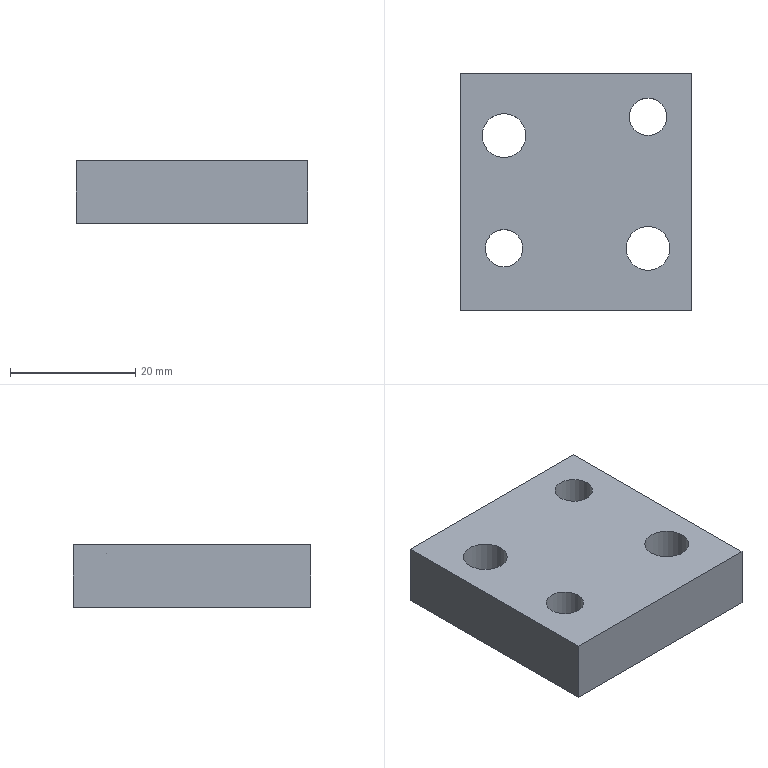Part | NX | features DIE-34 2 | 1 solid | 10 faces | box 37 x 38 x 10 mm | volume 12723 mm3 | plane 6 | cylinder 4 | commonest cylinder face diameters 6 x2 7.009 x2
STEP:
#1=CARTESIAN_POINT('',(2445.569,-956.622,868.716));
#2=VERTEX_POINT('',#1);
#3=CARTESIAN_POINT('',(2482.569,-956.622,868.716));
#4=VERTEX_POINT('',#3);
#5=CARTESIAN_POINT('',(2529.569,-956.622,868.716));
#6=DIRECTION('',(1.,0.,0.));
#7=VECTOR('',#6,1000.);
#8=LINE('',#5,#7);
#9=EDGE_CURVE('',#2,#4,#8,.T.);
#10=ORIENTED_EDGE('',*,*,#9,.T.);
#11=CARTESIAN_POINT('',(2482.569,-956.622,858.716));
#12=VERTEX_POINT('',#11);
#13=CARTESIAN_POINT('',(2482.569,-956.622,858.716));
#14=DIRECTION('',(0.,0.,1.));
#15=VECTOR('',#14,1000.);
#16=LINE('',#13,#15);
#17=EDGE_CURVE('',#4,#12,#16,.F.);
#18=ORIENTED_EDGE('',*,*,#17,.T.);
#19=CARTESIAN_POINT('',(2445.569,-956.622,858.716));
#20=VERTEX_POINT('',#19);
#21=CARTESIAN_POINT('',(2464.069,-956.622,858.716));
#22=DIRECTION('',(1.,0.,0.));
#23=VECTOR('',#22,1000.);
#24=LINE('',#21,#23);
#25=EDGE_CURVE('',#20,#12,#24,.T.);
#26=ORIENTED_EDGE('',*,*,#25,.F.);
#27=CARTESIAN_POINT('',(2445.569,-956.622,858.716));
#28=DIRECTION('',(0.,0.,1.));
#29=VECTOR('',#28,1000.);
#30=LINE('',#27,#29);
#31=EDGE_CURVE('',#20,#2,#30,.T.);
#32=ORIENTED_EDGE('',*,*,#31,.T.);
#33=EDGE_LOOP('',(#10,#18,#26,#32));
#34=FACE_BOUND('',#33,.T.);
#35=CARTESIAN_POINT('',(2464.069,-956.622,858.716));
#36=DIRECTION('',(0.,-1.,0.));
#37=DIRECTION('',(0.,0.,-1.));
#38=AXIS2_PLACEMENT_3D('',#35,#36,#37);
#39=PLANE('',#38);
#40=ADVANCED_FACE('',(#34),#39,.F.);
#41=CARTESIAN_POINT('',(2445.569,-994.622,868.716));
#42=VERTEX_POINT('',#41);
#43=CARTESIAN_POINT('',(2482.569,-994.622,868.716));
#44=VERTEX_POINT('',#43);
#45=CARTESIAN_POINT('',(2529.569,-994.622,868.716));
#46=DIRECTION('',(1.,0.,0.));
#47=VECTOR('',#46,1000.);
#48=LINE('',#45,#47);
#49=EDGE_CURVE('',#42,#44,#48,.T.);
#50=ORIENTED_EDGE('',*,*,#49,.F.);
#51=CARTESIAN_POINT('',(2445.569,-994.622,858.716));
#52=VERTEX_POINT('',#51);
#53=CARTESIAN_POINT('',(2445.569,-994.622,858.716));
#54=DIRECTION('',(0.,0.,1.));
#55=VECTOR('',#54,1000.);
#56=LINE('',#53,#55);
#57=EDGE_CURVE('',#52,#42,#56,.T.);
#58=ORIENTED_EDGE('',*,*,#57,.F.);
#59=CARTESIAN_POINT('',(2482.569,-994.622,858.716));
#60=VERTEX_POINT('',#59);
#61=CARTESIAN_POINT('',(2529.569,-994.622,858.716));
#62=DIRECTION('',(1.,0.,0.));
#63=VECTOR('',#62,1000.);
#64=LINE('',#61,#63);
#65=EDGE_CURVE('',#52,#60,#64,.T.);
#66=ORIENTED_EDGE('',*,*,#65,.T.);
#67=CARTESIAN_POINT('',(2482.569,-994.622,858.716));
#68=DIRECTION('',(0.,0.,1.));
#69=VECTOR('',#68,1000.);
#70=LINE('',#67,#69);
#71=EDGE_CURVE('',#44,#60,#70,.F.);
#72=ORIENTED_EDGE('',*,*,#71,.F.);
#73=EDGE_LOOP('',(#50,#58,#66,#72));
#74=FACE_BOUND('',#73,.T.);
#75=CARTESIAN_POINT('',(2529.569,-994.622,858.716));
#76=DIRECTION('',(0.,-1.,0.));
#77=DIRECTION('',(1.,0.,0.));
#78=AXIS2_PLACEMENT_3D('',#75,#76,#77);
#79=PLANE('',#78);
#80=ADVANCED_FACE('',(#74),#79,.T.);
#81=CARTESIAN_POINT('',(2456.073,-966.622,858.716));
#82=VERTEX_POINT('',#81);
#83=CARTESIAN_POINT('',(2452.569,-966.622,858.716));
#84=DIRECTION('',(0.,0.,1.));
#85=DIRECTION('',(1.,0.,0.));
#86=AXIS2_PLACEMENT_3D('',#83,#84,#85);
#87=CIRCLE('',#86,3.505);
#88=EDGE_CURVE('',#82,#82,#87,.T.);
#89=ORIENTED_EDGE('',*,*,#88,.F.);
#90=EDGE_LOOP('',(#89));
#91=FACE_BOUND('',#90,.T.);
#92=CARTESIAN_POINT('',(2456.073,-966.622,868.716));
#93=VERTEX_POINT('',#92);
#94=CARTESIAN_POINT('',(2452.569,-966.622,868.716));
#95=DIRECTION('',(0.,0.,1.));
#96=DIRECTION('',(1.,0.,0.));
#97=AXIS2_PLACEMENT_3D('',#94,#95,#96);
#98=CIRCLE('',#97,3.505);
#99=EDGE_CURVE('',#93,#93,#98,.T.);
#100=ORIENTED_EDGE('',*,*,#99,.T.);
#101=EDGE_LOOP('',(#100));
#102=FACE_BOUND('',#101,.T.);
#103=CARTESIAN_POINT('',(2452.569,-966.622,858.716));
#104=DIRECTION('',(0.,0.,1.));
#105=DIRECTION('',(1.,0.,0.));
#106=AXIS2_PLACEMENT_3D('',#103,#104,#105);
#107=CYLINDRICAL_SURFACE('',#106,3.505);
#108=ADVANCED_FACE('',(#91,#102),#107,.F.);
#109=CARTESIAN_POINT('',(2455.569,-984.622,858.716));
#110=VERTEX_POINT('',#109);
#111=CARTESIAN_POINT('',(2452.569,-984.622,858.716));
#112=DIRECTION('',(0.,0.,1.));
#113=DIRECTION('',(1.,0.,0.));
#114=AXIS2_PLACEMENT_3D('',#111,#112,#113);
#115=CIRCLE('',#114,3.);
#116=EDGE_CURVE('',#110,#110,#115,.T.);
#117=ORIENTED_EDGE('',*,*,#116,.F.);
#118=EDGE_LOOP('',(#117));
#119=FACE_BOUND('',#118,.T.);
#120=CARTESIAN_POINT('',(2455.569,-984.622,868.716));
#121=VERTEX_POINT('',#120);
#122=CARTESIAN_POINT('',(2452.569,-984.622,868.716));
#123=DIRECTION('',(0.,0.,1.));
#124=DIRECTION('',(1.,0.,0.));
#125=AXIS2_PLACEMENT_3D('',#122,#123,#124);
#126=CIRCLE('',#125,3.);
#127=EDGE_CURVE('',#121,#121,#126,.T.);
#128=ORIENTED_EDGE('',*,*,#127,.T.);
#129=EDGE_LOOP('',(#128));
#130=FACE_BOUND('',#129,.T.);
#131=CARTESIAN_POINT('',(2452.569,-984.622,858.716));
#132=DIRECTION('',(0.,0.,1.));
#133=DIRECTION('',(1.,0.,0.));
#134=AXIS2_PLACEMENT_3D('',#131,#132,#133);
#135=CYLINDRICAL_SURFACE('',#134,3.);
#136=ADVANCED_FACE('',(#119,#130),#135,.F.);
#137=CARTESIAN_POINT('',(2445.569,-849.622,868.716));
#138=DIRECTION('',(0.,1.,0.));
#139=VECTOR('',#138,1000.);
#140=LINE('',#137,#139);
#141=EDGE_CURVE('',#42,#2,#140,.T.);
#142=ORIENTED_EDGE('',*,*,#141,.T.);
#143=ORIENTED_EDGE('',*,*,#31,.F.);
#144=CARTESIAN_POINT('',(2445.569,-989.622,858.716));
#145=DIRECTION('',(0.,1.,0.));
#146=VECTOR('',#145,1000.);
#147=LINE('',#144,#146);
#148=EDGE_CURVE('',#52,#20,#147,.T.);
#149=ORIENTED_EDGE('',*,*,#148,.F.);
#150=ORIENTED_EDGE('',*,*,#57,.T.);
#151=EDGE_LOOP('',(#142,#143,#149,#150));
#152=FACE_BOUND('',#151,.T.);
#153=CARTESIAN_POINT('',(2445.569,-989.622,858.716));
#154=DIRECTION('',(1.,0.,0.));
#155=DIRECTION('',(0.,0.,-1.));
#156=AXIS2_PLACEMENT_3D('',#153,#154,#155);
#157=PLANE('',#156);
#158=ADVANCED_FACE('',(#152),#157,.F.);
#159=ORIENTED_EDGE('',*,*,#116,.T.);
#160=EDGE_LOOP('',(#159));
#161=FACE_BOUND('',#160,.T.);
#162=ORIENTED_EDGE('',*,*,#88,.T.);
#163=EDGE_LOOP('',(#162));
#164=FACE_BOUND('',#163,.T.);
#165=ORIENTED_EDGE('',*,*,#25,.T.);
#166=CARTESIAN_POINT('',(2482.569,-989.622,858.716));
#167=DIRECTION('',(0.,-1.,0.));
#168=VECTOR('',#167,1000.);
#169=LINE('',#166,#168);
#170=EDGE_CURVE('',#60,#12,#169,.F.);
#171=ORIENTED_EDGE('',*,*,#170,.F.);
#172=ORIENTED_EDGE('',*,*,#65,.F.);
#173=ORIENTED_EDGE('',*,*,#148,.T.);
#174=EDGE_LOOP('',(#165,#171,#172,#173));
#175=FACE_BOUND('',#174,.T.);
#176=CARTESIAN_POINT('',(2478.569,-963.622,858.716));
#177=VERTEX_POINT('',#176);
#178=CARTESIAN_POINT('',(2475.569,-963.622,858.716));
#179=DIRECTION('',(0.,0.,1.));
#180=DIRECTION('',(1.,0.,0.));
#181=AXIS2_PLACEMENT_3D('',#178,#179,#180);
#182=CIRCLE('',#181,3.);
#183=EDGE_CURVE('',#177,#177,#182,.F.);
#184=ORIENTED_EDGE('',*,*,#183,.F.);
#185=EDGE_LOOP('',(#184));
#186=FACE_BOUND('',#185,.T.);
#187=CARTESIAN_POINT('',(2479.073,-984.622,858.716));
#188=VERTEX_POINT('',#187);
#189=CARTESIAN_POINT('',(2475.569,-984.622,858.716));
#190=DIRECTION('',(0.,0.,1.));
#191=DIRECTION('',(1.,0.,0.));
#192=AXIS2_PLACEMENT_3D('',#189,#190,#191);
#193=CIRCLE('',#192,3.505);
#194=EDGE_CURVE('',#188,#188,#193,.F.);
#195=ORIENTED_EDGE('',*,*,#194,.F.);
#196=EDGE_LOOP('',(#195));
#197=FACE_BOUND('',#196,.T.);
#198=CARTESIAN_POINT('',(2529.569,-849.622,858.716));
#199=DIRECTION('',(0.,0.,1.));
#200=DIRECTION('',(-1.,0.,0.));
#201=AXIS2_PLACEMENT_3D('',#198,#199,#200);
#202=PLANE('',#201);
#203=ADVANCED_FACE('',(#161,#164,#175,#186,#197),#202,.F.);
#204=ORIENTED_EDGE('',*,*,#127,.F.);
#205=EDGE_LOOP('',(#204));
#206=FACE_BOUND('',#205,.T.);
#207=ORIENTED_EDGE('',*,*,#99,.F.);
#208=EDGE_LOOP('',(#207));
#209=FACE_BOUND('',#208,.T.);
#210=ORIENTED_EDGE('',*,*,#9,.F.);
#211=ORIENTED_EDGE('',*,*,#141,.F.);
#212=ORIENTED_EDGE('',*,*,#49,.T.);
#213=CARTESIAN_POINT('',(2482.569,-989.622,868.716));
#214=DIRECTION('',(0.,1.,0.));
#215=VECTOR('',#214,1000.);
#216=LINE('',#213,#215);
#217=EDGE_CURVE('',#44,#4,#216,.T.);
#218=ORIENTED_EDGE('',*,*,#217,.T.);
#219=EDGE_LOOP('',(#210,#211,#212,#218));
#220=FACE_BOUND('',#219,.T.);
#221=CARTESIAN_POINT('',(2478.569,-963.622,868.716));
#222=VERTEX_POINT('',#221);
#223=CARTESIAN_POINT('',(2475.569,-963.622,868.716));
#224=DIRECTION('',(0.,0.,1.));
#225=DIRECTION('',(1.,0.,0.));
#226=AXIS2_PLACEMENT_3D('',#223,#224,#225);
#227=CIRCLE('',#226,3.);
#228=EDGE_CURVE('',#222,#222,#227,.F.);
#229=ORIENTED_EDGE('',*,*,#228,.T.);
#230=EDGE_LOOP('',(#229));
#231=FACE_BOUND('',#230,.T.);
#232=CARTESIAN_POINT('',(2479.073,-984.622,868.716));
#233=VERTEX_POINT('',#232);
#234=CARTESIAN_POINT('',(2475.569,-984.622,868.716));
#235=DIRECTION('',(0.,0.,1.));
#236=DIRECTION('',(1.,0.,0.));
#237=AXIS2_PLACEMENT_3D('',#234,#235,#236);
#238=CIRCLE('',#237,3.505);
#239=EDGE_CURVE('',#233,#233,#238,.F.);
#240=ORIENTED_EDGE('',*,*,#239,.T.);
#241=EDGE_LOOP('',(#240));
#242=FACE_BOUND('',#241,.T.);
#243=CARTESIAN_POINT('',(2529.569,-849.622,868.716));
#244=DIRECTION('',(0.,0.,1.));
#245=DIRECTION('',(-1.,0.,0.));
#246=AXIS2_PLACEMENT_3D('',#243,#244,#245);
#247=PLANE('',#246);
#248=ADVANCED_FACE('',(#206,#209,#220,#231,#242),#247,.T.);
#249=ORIENTED_EDGE('',*,*,#217,.F.);
#250=ORIENTED_EDGE('',*,*,#71,.T.);
#251=ORIENTED_EDGE('',*,*,#170,.T.);
#252=ORIENTED_EDGE('',*,*,#17,.F.);
#253=EDGE_LOOP('',(#249,#250,#251,#252));
#254=FACE_BOUND('',#253,.T.);
#255=CARTESIAN_POINT('',(2482.569,-989.622,858.716));
#256=DIRECTION('',(-1.,0.,0.));
#257=DIRECTION('',(0.,0.,1.));
#258=AXIS2_PLACEMENT_3D('',#255,#256,#257);
#259=PLANE('',#258);
#260=ADVANCED_FACE('',(#254),#259,.F.);
#261=ORIENTED_EDGE('',*,*,#194,.T.);
#262=EDGE_LOOP('',(#261));
#263=FACE_BOUND('',#262,.T.);
#264=ORIENTED_EDGE('',*,*,#239,.F.);
#265=EDGE_LOOP('',(#264));
#266=FACE_BOUND('',#265,.T.);
#267=CARTESIAN_POINT('',(2475.569,-984.622,858.716));
#268=DIRECTION('',(0.,0.,1.));
#269=DIRECTION('',(1.,0.,0.));
#270=AXIS2_PLACEMENT_3D('',#267,#268,#269);
#271=CYLINDRICAL_SURFACE('',#270,3.505);
#272=ADVANCED_FACE('',(#263,#266),#271,.F.);
#273=ORIENTED_EDGE('',*,*,#183,.T.);
#274=EDGE_LOOP('',(#273));
#275=FACE_BOUND('',#274,.T.);
#276=ORIENTED_EDGE('',*,*,#228,.F.);
#277=EDGE_LOOP('',(#276));
#278=FACE_BOUND('',#277,.T.);
#279=CARTESIAN_POINT('',(2475.569,-963.622,858.716));
#280=DIRECTION('',(0.,0.,1.));
#281=DIRECTION('',(1.,0.,0.));
#282=AXIS2_PLACEMENT_3D('',#279,#280,#281);
#283=CYLINDRICAL_SURFACE('',#282,3.);
#284=ADVANCED_FACE('',(#275,#278),#283,.F.);
#285=CLOSED_SHELL('',(#40,#80,#108,#136,#158,#203,#248,#260,#272,#284));
#286=MANIFOLD_SOLID_BREP('',#285);
#287=(LENGTH_UNIT()NAMED_UNIT(*)SI_UNIT(.MILLI.,.METRE.));
#288=UNCERTAINTY_MEASURE_WITH_UNIT(LENGTH_MEASURE(0.00001),#287,'','');
#289=(NAMED_UNIT(*)PLANE_ANGLE_UNIT()SI_UNIT($,.RADIAN.));
#290=(NAMED_UNIT(*)SI_UNIT($,.STERADIAN.)SOLID_ANGLE_UNIT());
#291=(GEOMETRIC_REPRESENTATION_CONTEXT(3)GLOBAL_UNCERTAINTY_ASSIGNED_CONTEXT((#288))GLOBAL_UNIT_ASSIGNED_CONTEXT((#287,#289,#290))REPRESENTATION_CONTEXT('',''));
#292=ADVANCED_BREP_SHAPE_REPRESENTATION('',(#286),#291);